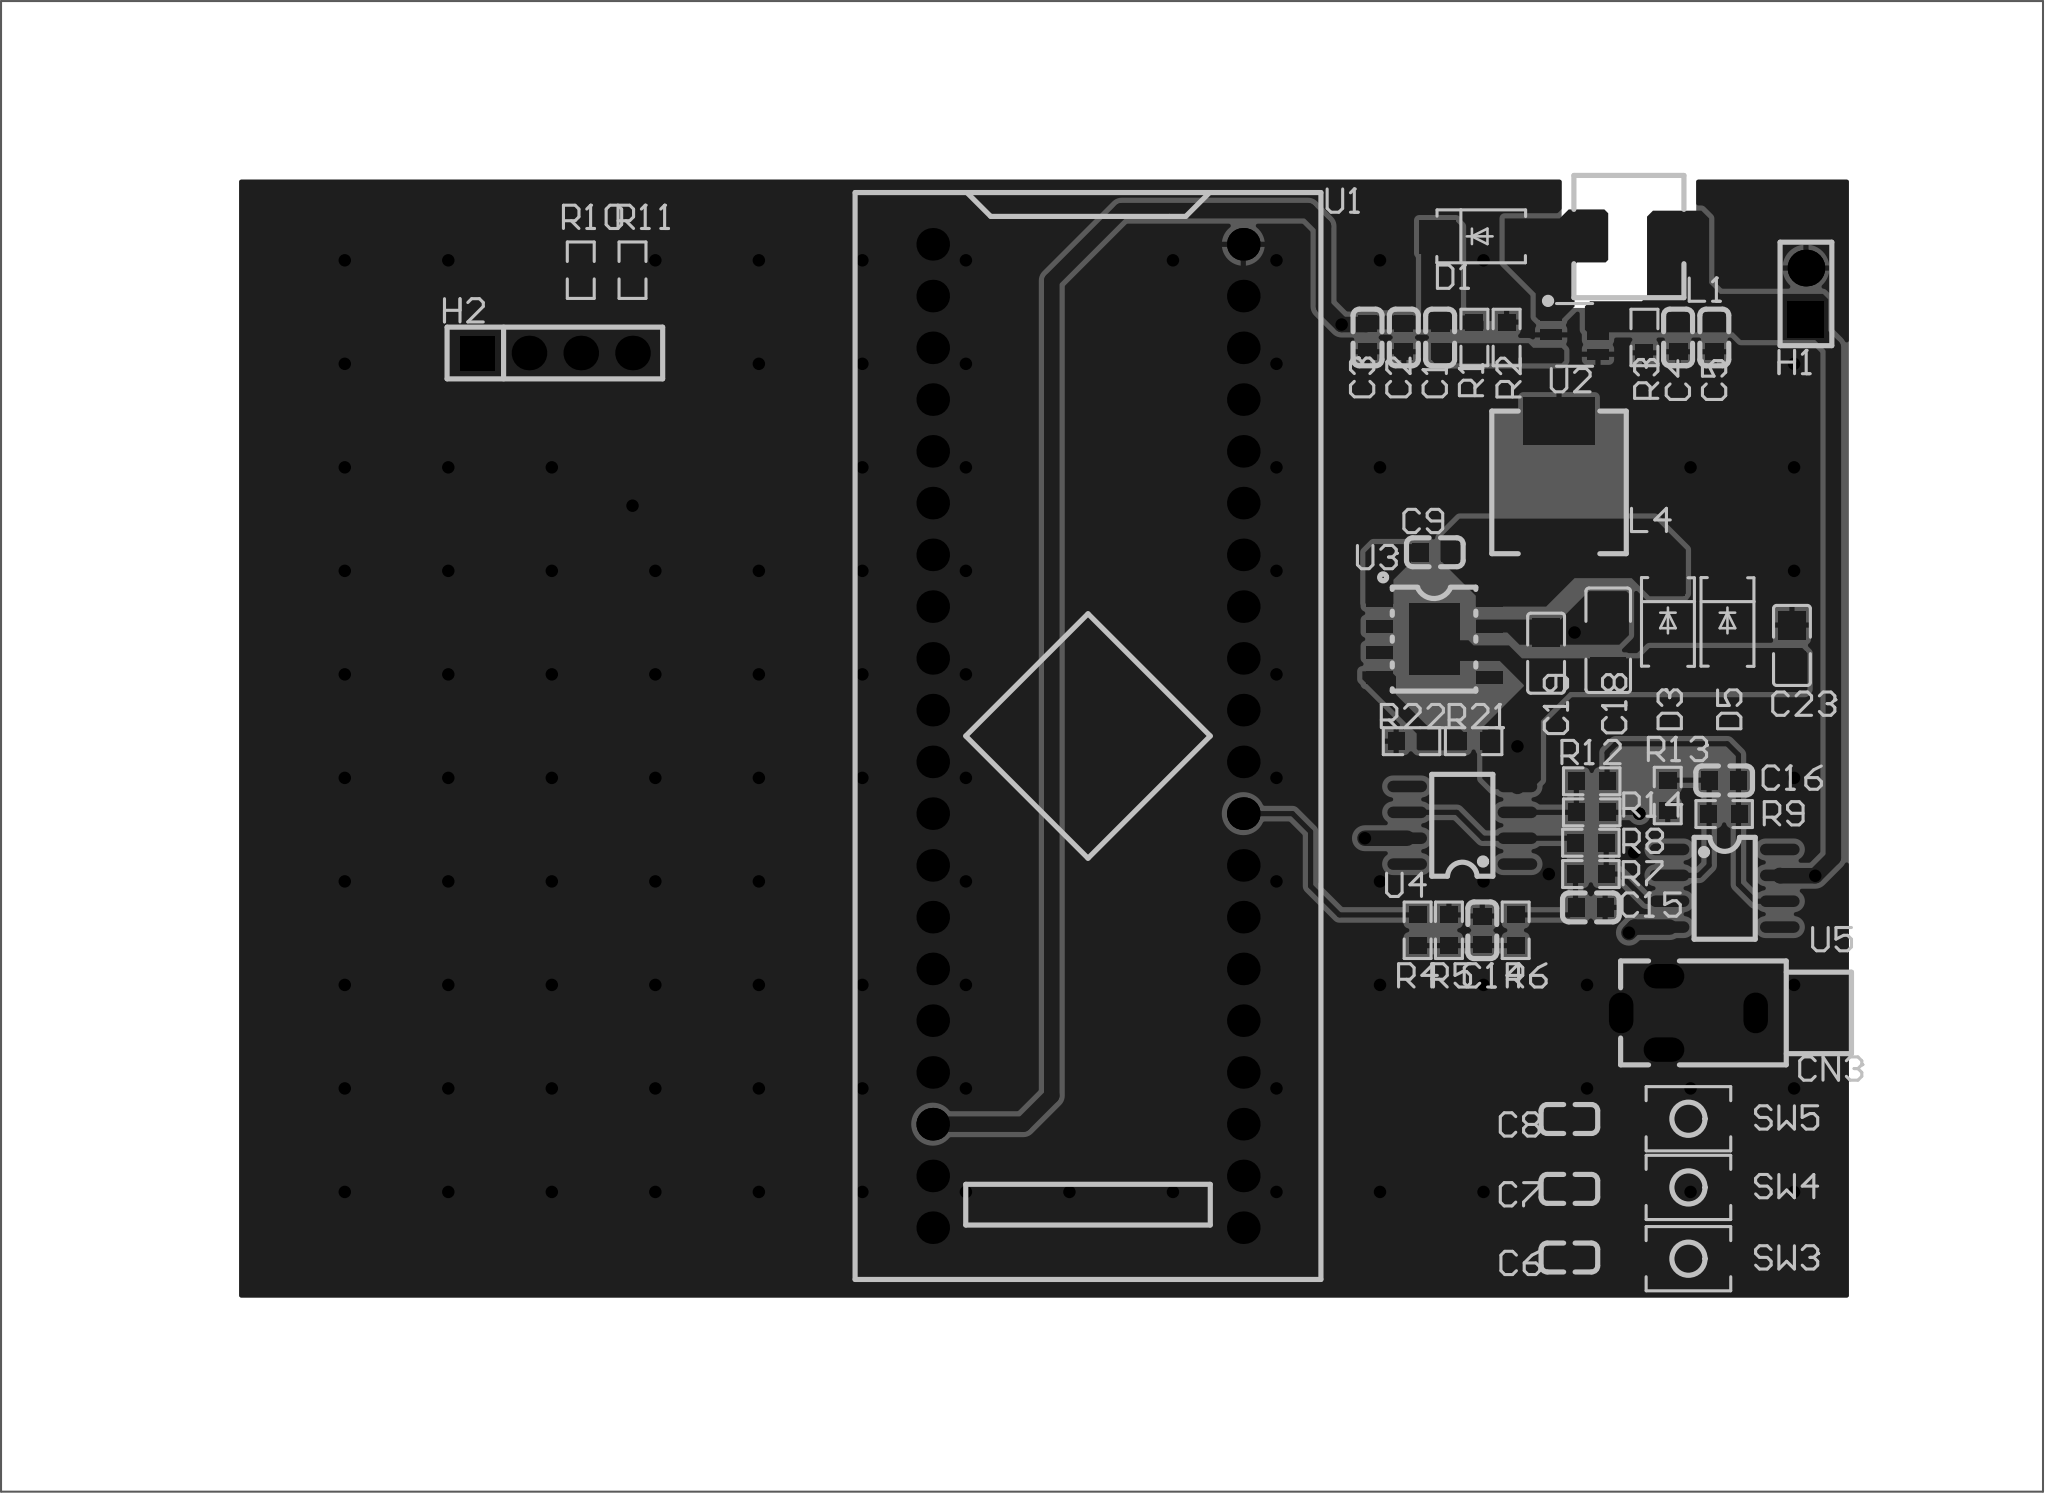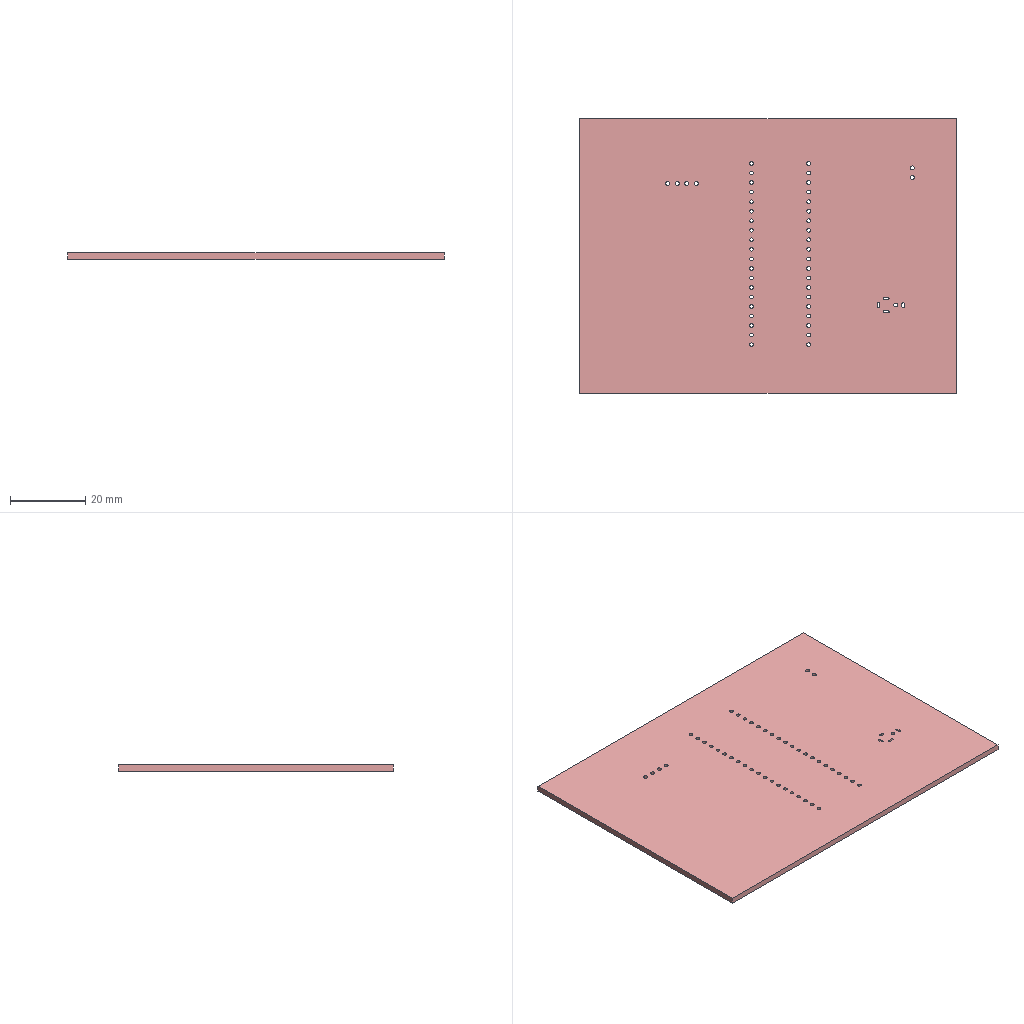Circuit board layout | Altium Designer | box 100.2 x 73.2 x 1.6 mm
Layer stack:
# Altium Designer layer stack of  (unit mm; dielectric type: 0 none, 1 core, 2 prepreg, 3 surface material)
index,name,kind,layer,copper_thickness_mm,dielectric_type,dielectric_thickness_mm,dielectric_material,dielectric_constant
0,Top Paste Mask Layer,other,,,,,,
1,Top Silkscreen Layer,other,,,,,,
2,Top Solder Mask Layer,dielectric,,,3,0.01,,3.3
3,Top Layer,copper,Top Layer,0.035,,,,
4,Dielectric1,dielectric,,,3,1.51,FR4,4.5
5,Bottom Layer,copper,Bottom Layer,0.035,,,,
6,Bottom Solder Mask Layer,dielectric,,,3,0.01,,3.3
7,Bottom Silkscreen Layer,other,,,,,,
8,Bottom Paste Mask Layer,other,,,,,,
# drill layer pairs: low layer,high layer
drill_pair,Top Layer,Bottom Layer
Part placement:
Designator,Comment,Layer,Footprint,Center-X(mm),Center-Y(mm),Rotation
C6,10uF,TopLayer,C0603,146.812,81.341,180
C7,10uF,TopLayer,C0603,146.812,84.709,180
C8,10uF,TopLayer,C0603,146.812,88.138,180
C14,47uF,TopLayer,C0603,142.538,97.4,90
C15,47uF,TopLayer,C0603,147.866,98.522,0
C16,510pF,TopLayer,C0603,154.407,104.754,0
CN3,PJ-210B,TopLayer,AUDIO-TH_PJ-210B,152.654,93.345,90
R4,3.3K,TopLayer,R0603,139.364,97.4,270
R5,5.1K,TopLayer,R0603,140.901,97.4,90
R6,2.2K,TopLayer,R0603,144.175,97.4,270
R7,1K,TopLayer,R0603,147.866,100.159,0
R8,1K,TopLayer,R0603,147.866,101.696,180
R9,1K,TopLayer,R0603,154.407,103.103,0
R10,4.7K,TopLayer,R0603,98.298,129.794,270
R11,4.7K,TopLayer,R0603,100.838,129.794,270
R12,10K,TopLayer,R0603,147.908,104.712,0
R13,1K,TopLayer,R0603,151.638,104.013,90
R14,1K,TopLayer,R0603,147.908,103.188,180
SW3,,TopLayer,Key_SMD_3x4x2,152.654,81.283,0
SW4,,TopLayer,Key_SMD_3x4x2,152.654,84.78,0
SW5,,TopLayer,Key_SMD_3x4x2,152.654,88.15,0
U1,STM32F103C8T6-Card,TopLayer,CONN-TH_L53.3-W22.9_STM32F103C8T6-CARD,123.19,106.934,270
U4,OPA140AIDR,TopLayer,SOIC-8_L5.0-W4.0-P1.27-LS6.0-BL,141.558,102.553,90
U5,OPA140AIDR,TopLayer,SOIC-8_L5.0-W4.0-P1.27-LS6.0-BL,154.432,99.461,270
H2,,TopLayer,HDR-TH_4P-P2.54-V-F,97.028,125.73,0
C1,22pF,TopLayer,C0603,140.469,126.492,90
C2,1uF,TopLayer,C0603,138.688,126.492,90
C3,22uF,TopLayer,C0603,136.906,126.492,90
C4,1uF,TopLayer,C0603,152.146,126.492,90
C5,22uF,TopLayer,C0603,153.924,126.492,90
C9,100nF,TopLayer,C0603,140.208,115.951,0
C18,10uF,TopLayer,C1206,148.717,111.633,90
C19,100nF,TopLayer,C0805,145.669,110.998,90
C23,22uF,TopLayer,C0805,157.734,111.379,90
D1,SS34,TopLayer,SMA_L4.3-W2.6-LS5.0-FD,142.494,131.445,180
D3,SS34,TopLayer,SMA_L4.3-W2.6-LS5.0-FD,151.638,112.522,90
D5,SS34,TopLayer,SMA_L4.3-W2.6-LS5.0-FD,154.559,112.522,90
L1,10uH,TopLayer,IND-SMD_L6.0-W5.2_SUMIDA_CDH53,149.733,131.445,90
L4,10uH,TopLayer,IND-SMD_L7.3-W6.8,146.304,119.38,90
R1,39kΩ,TopLayer,R0603,142.151,126.492,90
R2,10kΩ,TopLayer,R0603,143.732,126.492,270
R3,100kΩ,TopLayer,R0603,150.495,126.492,90
R21,15.8kΩ,TopLayer,R0603,142.113,106.68,180
R22,140kΩ,TopLayer,R0603,139.065,106.68,180
U2,MT3608,TopLayer,SOT-23-6_L2.9-W1.6-P0.95-LS2.8-BL,147.066,126.619,270
U3,TPS5430DDAR,TopLayer,ESOP-8_L4.9-W3.9-P1.27-LS6.0-TL-EP,140.171,111.689,0
H1,,TopLayer,HDR-TH_2P-P2.54-V-M-1,158.421,128.629,90
Pad and via stacks:
# Altium Designer via and pad stacks of  (unit mm). Each distinct definition once, with the count of objects using it.
# via: kind,start_layer,end_layer,hole_mm,diameter_mm,mode(0 simple;1 top-mid-bottom;2 full stack),diameter_per_layer,count,example_net
# pad: kind,layer,hole_mm,hole_type(0 round;1 square;2 slot),plating,top_size,top_shape(1 round;2 rect;3 octagon;9 rounded rect),mid_size,bottom_size,mode,footprint,size_per_layer,count,example
pad,Top Layer,0,0,plated,0.8x0.9,2,0.8x0.9,0.8x0.9,0,C0603,,24,C6.2
pad,Top Layer,0,0,plated,0.8065x0.864,2,0.8065x0.864,0.8065x0.864,0,R0603,,32,R4.2
pad,Top Layer,0,0,plated,1.53x1.36,2,1.53x1.36,1.53x1.36,0,Key_SMD_3x4x2,,6,SW3.1
pad,Top Layer,0,0,plated,0.5684x1.95,1,0.5684x1.95,0.5684x1.95,0,SOIC-8_L5.0-W4.0-P1.27-LS6.0-BL,,16,U4.1
pad,Top Layer,0,0,plated,1.485x1.728,2,1.485x1.728,1.485x1.728,0,C1206,,2,C18.2
pad,Top Layer,0,0,plated,1.41x1.35,2,1.41x1.35,1.41x1.35,0,C0805,,4,C19.2
pad,Top Layer,0,0,plated,1.8x1.62,2,1.8x1.62,1.8x1.62,0,SMA_L4.3-W2.6-LS5.0-FD,,2,D1.1
pad,Top Layer,0,0,plated,2.046x1.62,2,2.046x1.62,2.046x1.62,0,SMA_L4.3-W2.6-LS5.0-FD,,4,D3.1
pad,Top Layer,0,0,plated,2.2x1.75,2,2.2x1.75,2.2x1.75,0,IND-SMD_L6.0-W5.2_SUMIDA_CDH53,,2,L1.2
pad,Top Layer,0,0,plated,2.35x3.5,2,2.35x3.5,2.35x3.5,0,IND-SMD_L7.3-W6.8,,2,L4.2
pad,Top Layer,0,0,plated,0.532x1.072,2,0.532x1.072,0.532x1.072,0,SOT-23-6_L2.9-W1.6-P0.95-LS2.8-BL,,6,U2.1
pad,Top Layer,0,0,plated,1.3x0.6,2,1.3x0.6,1.3x0.6,0,ESOP-8_L4.9-W3.9-P1.27-LS6.0-TL-EP,,8,U3.1
pad,Top Layer,0,0,plated,2.5x3.5,2,2.5x3.5,2.5x3.5,0,ESOP-8_L4.9-W3.9-P1.27-LS6.0-TL-EP,,1,U3.9
pad,Multi-Layer,0.6,2,plated,1.2x2,1,1.2x2,1.2x2,0,AUDIO-TH_PJ-210B,,4,CN3.1
pad,Multi-Layer,1,0,plated,1.6x1.6,1,1.6x1.6,1.6x1.6,0,CONN-TH_L53.3-W22.9_STM32F103C8T6-CARD,,40,U1.1
pad,Multi-Layer,1.1,0,plated,1.7x1.7,2,1.7x1.7,1.7x1.7,0,HDR-TH_4P-P2.54-V-F,,1,H2.1
pad,Multi-Layer,1.1,0,plated,1.7x1.7,1,1.7x1.7,1.7x1.7,0,HDR-TH_4P-P2.54-V-F,,3,H2.2
pad,Multi-Layer,1.1,0,plated,1.8x1.8,1,1.8x1.8,1.8x1.8,0,HDR-TH_2P-P2.54-V-M-1,,1,H1.2
pad,Multi-Layer,1.1,0,plated,1.8x1.8,2,1.8x1.8,1.8x1.8,0,HDR-TH_2P-P2.54-V-M-1,,1,H1.1
via,Top Layer,Bottom Layer,0.3048,0.61,0,,106,PB7
Copper pours:
name,layer,net,type(0 solid;1 hatched;2 none)
Top Layer-GND,Top Layer,GND,0
Bottom Layer-GND,Bottom Layer,GND,0
Design rules, without the lines most boards share:
# Altium Designer design rules of  (exported by Altium Designer, unit mm)
# columns: name | kind | enabled | priority | scope1 | scope2 | descriptor | typed fields (field=value)
creepage | 65 | enabled | 1 | All | All | Creepage Distance Constraint =(0mil) (All),(All) |
copperRegion | 20 | enabled | 1 | (InNet('GND')) | All | Polygon Connect Rule(Relief Connect )(Conductor Width=10mil) (Relief Angle=90 Angle) (Entries=4) (Air Gap Width=10mil) ((InNet('GND'))),(All) | connect_style(0=relief,1=direct,2=none)=0 relief_conductor_width=0.254 relief_entries=4